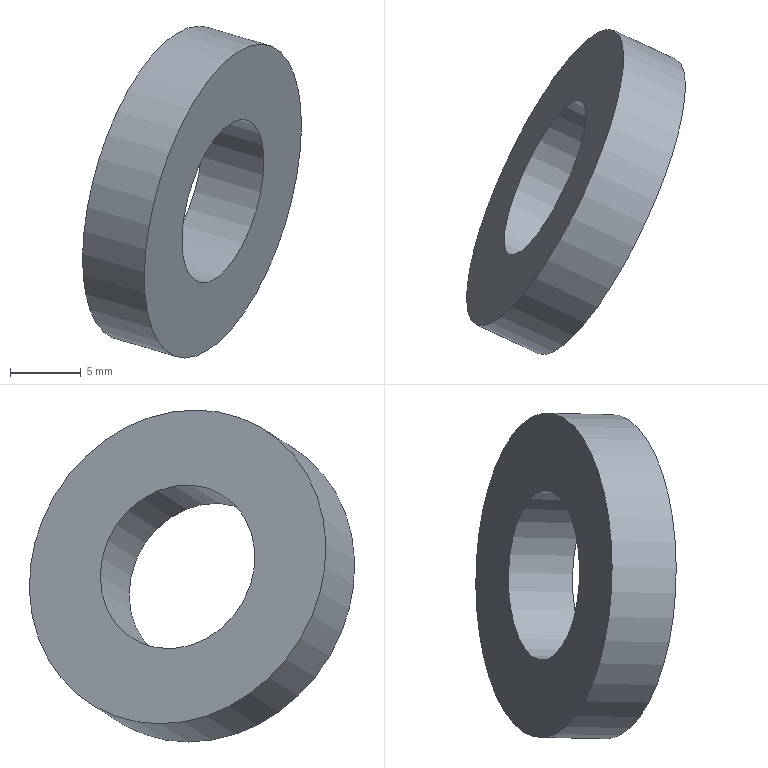Part | NX | features solid 2 | 1 solid | 4 faces | box 15.494 x 23.037 x 23.51 mm | volume 1512 mm3 | cylinder 2 | plane 2 | commonest cylinder face diameters 12 x1 23 x1
STEP:
#1=CARTESIAN_POINT('',(-844.318,752.529,-107.047));
#2=VERTEX_POINT('',#1);
#3=CARTESIAN_POINT('',(-839.458,762.952,-107.047));
#4=DIRECTION('',(-0.8754,0.4082,0.2588));
#5=DIRECTION('',(-0.4226,-0.9063,-0.000000003));
#6=AXIS2_PLACEMENT_3D('',#3,#4,#5);
#7=CIRCLE('',#6,11.5);
#8=EDGE_CURVE('',#2,#2,#7,.F.);
#9=ORIENTED_EDGE('',*,*,#8,.T.);
#10=EDGE_LOOP('',(#9));
#11=FACE_BOUND('',#10,.T.);
#12=CARTESIAN_POINT('',(-839.941,750.488,-108.341));
#13=VERTEX_POINT('',#12);
#14=CARTESIAN_POINT('',(-835.08,760.911,-108.341));
#15=DIRECTION('',(-0.8754,0.4082,0.2588));
#16=DIRECTION('',(-0.4226,-0.9063,-0.000000003));
#17=AXIS2_PLACEMENT_3D('',#14,#15,#16);
#18=CIRCLE('',#17,11.5);
#19=EDGE_CURVE('',#13,#13,#18,.F.);
#20=ORIENTED_EDGE('',*,*,#19,.F.);
#21=EDGE_LOOP('',(#20));
#22=FACE_BOUND('',#21,.T.);
#23=CARTESIAN_POINT('',(-835.08,760.911,-108.341));
#24=DIRECTION('',(-0.8754,0.4082,0.2588));
#25=DIRECTION('',(-0.4226,-0.9063,-0.000000003));
#26=AXIS2_PLACEMENT_3D('',#23,#24,#25);
#27=CYLINDRICAL_SURFACE('',#26,11.5);
#28=ADVANCED_FACE('',(#11,#22),#27,.T.);
#29=ORIENTED_EDGE('',*,*,#19,.T.);
#30=EDGE_LOOP('',(#29));
#31=FACE_BOUND('',#30,.T.);
#32=CARTESIAN_POINT('',(-837.616,755.473,-108.341));
#33=VERTEX_POINT('',#32);
#34=CARTESIAN_POINT('',(-835.08,760.911,-108.341));
#35=DIRECTION('',(-0.8754,0.4082,0.2588));
#36=DIRECTION('',(-0.4226,-0.9063,-0.000000003));
#37=AXIS2_PLACEMENT_3D('',#34,#35,#36);
#38=CIRCLE('',#37,6.);
#39=EDGE_CURVE('',#33,#33,#38,.F.);
#40=ORIENTED_EDGE('',*,*,#39,.F.);
#41=EDGE_LOOP('',(#40));
#42=FACE_BOUND('',#41,.T.);
#43=CARTESIAN_POINT('',(-835.08,760.911,-108.341));
#44=DIRECTION('',(-0.8754,0.4082,0.2588));
#45=DIRECTION('',(-0.4226,-0.9063,-0.000000003));
#46=AXIS2_PLACEMENT_3D('',#43,#44,#45);
#47=PLANE('',#46);
#48=ADVANCED_FACE('',(#31,#42),#47,.F.);
#49=ORIENTED_EDGE('',*,*,#8,.F.);
#50=EDGE_LOOP('',(#49));
#51=FACE_BOUND('',#50,.T.);
#52=CARTESIAN_POINT('',(-841.993,757.514,-107.047));
#53=VERTEX_POINT('',#52);
#54=CARTESIAN_POINT('',(-839.458,762.952,-107.047));
#55=DIRECTION('',(-0.8754,0.4082,0.2588));
#56=DIRECTION('',(-0.4226,-0.9063,-0.000000003));
#57=AXIS2_PLACEMENT_3D('',#54,#55,#56);
#58=CIRCLE('',#57,6.);
#59=EDGE_CURVE('',#53,#53,#58,.F.);
#60=ORIENTED_EDGE('',*,*,#59,.T.);
#61=EDGE_LOOP('',(#60));
#62=FACE_BOUND('',#61,.T.);
#63=CARTESIAN_POINT('',(-839.458,762.952,-107.047));
#64=DIRECTION('',(-0.8754,0.4082,0.2588));
#65=DIRECTION('',(-0.4226,-0.9063,-0.000000003));
#66=AXIS2_PLACEMENT_3D('',#63,#64,#65);
#67=PLANE('',#66);
#68=ADVANCED_FACE('',(#51,#62),#67,.T.);
#69=ORIENTED_EDGE('',*,*,#59,.F.);
#70=EDGE_LOOP('',(#69));
#71=FACE_BOUND('',#70,.T.);
#72=ORIENTED_EDGE('',*,*,#39,.T.);
#73=EDGE_LOOP('',(#72));
#74=FACE_BOUND('',#73,.T.);
#75=CARTESIAN_POINT('',(-835.08,760.911,-108.341));
#76=DIRECTION('',(-0.8754,0.4082,0.2588));
#77=DIRECTION('',(-0.4226,-0.9063,-0.000000003));
#78=AXIS2_PLACEMENT_3D('',#75,#76,#77);
#79=CYLINDRICAL_SURFACE('',#78,6.);
#80=ADVANCED_FACE('',(#71,#74),#79,.F.);
#81=CLOSED_SHELL('',(#28,#48,#68,#80));
#82=MANIFOLD_SOLID_BREP('',#81);
#83=(LENGTH_UNIT()NAMED_UNIT(*)SI_UNIT(.MILLI.,.METRE.));
#84=UNCERTAINTY_MEASURE_WITH_UNIT(LENGTH_MEASURE(0.00001),#83,'','');
#85=(NAMED_UNIT(*)PLANE_ANGLE_UNIT()SI_UNIT($,.RADIAN.));
#86=(NAMED_UNIT(*)SI_UNIT($,.STERADIAN.)SOLID_ANGLE_UNIT());
#87=(GEOMETRIC_REPRESENTATION_CONTEXT(3)GLOBAL_UNCERTAINTY_ASSIGNED_CONTEXT((#84))GLOBAL_UNIT_ASSIGNED_CONTEXT((#83,#85,#86))REPRESENTATION_CONTEXT('',''));
#88=ADVANCED_BREP_SHAPE_REPRESENTATION('',(#82),#87);